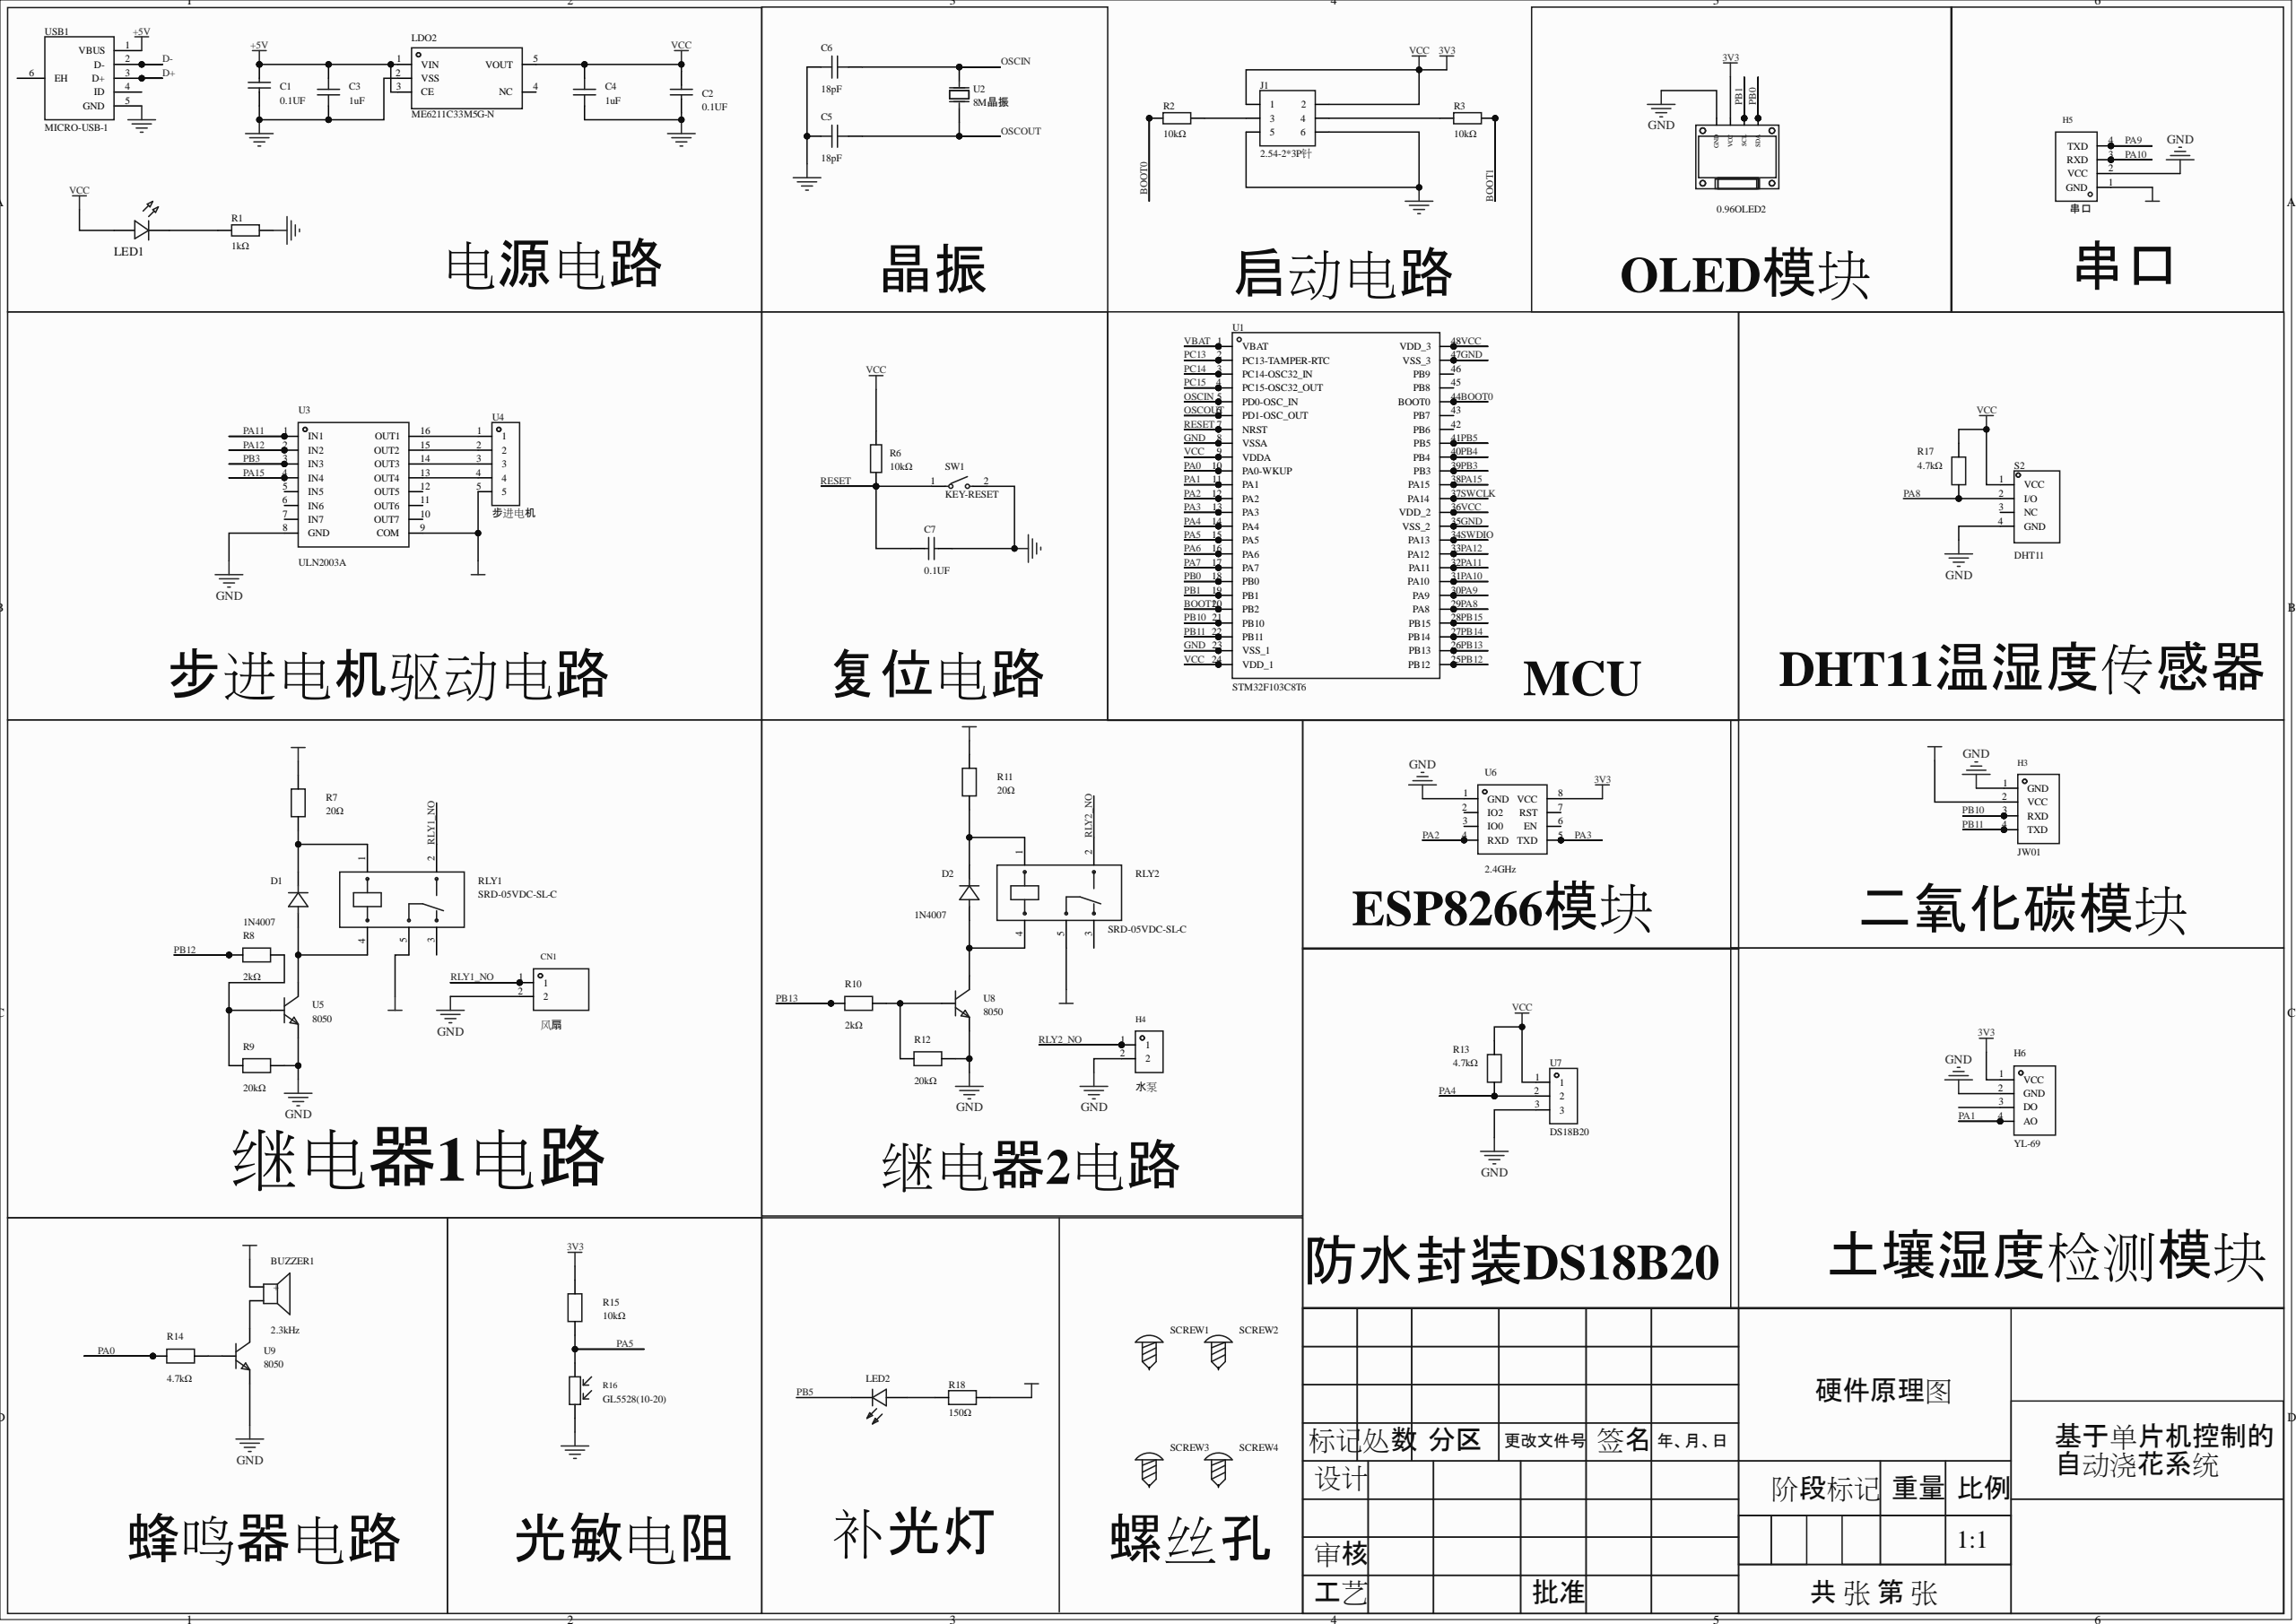Circuit board | Altium Designer | 54 parts | 46 nets
Bill of materials:
Comment,Description,Designator,Footprint,LibRef,Quantity
"","","0.96OLED2","oled-th_l27.8-w27.2-p2.54_c9900033791","0.96OLED模块_4P","1"
"2.3kHz","","BUZZER1","BUZ-TH_BD12.0-P7.60-D0.6-FD","TMB12A05_C96093","1"
"0.1UF","","C1, C2, C7","C0603","CAPCER0.1UF16VX5R0603,CAPCER0.1UF25VX5R0603,CAPCER0.1UF16VX7R0603","3"
"1uF","","C3, C4","C0603","TMK107B7105MA-T","2"
"18pF","","C5, C6","C0603","C1608C0G1H180J080AA","2"
"风扇","","CN1","CONN-TH_B2B-XH-A-LF-SN","B2B-XH-A(LF)(SN)","1"
"1N4007","","D1, D2","DO-41_BD2.4-L4.7-P8.70-D0.8-RD","1N4007_C2985028","2"
"JW01","","H3","HDR-TH_4P-P2.54-V-M","PZ254V-11-04P","1"
"水泵","","H4","HDR-TH_2P-P2.54-V-M","PZ254V-11-02P","1"
"串口","","H5","HDR-TH_4P-P2.54-V-M","PZ254V-11-04P","1"
"YL-69","","H6","HDR-TH_4P-P2.54-V-F","PM254V-11-04-H85","1"
"2.54-2*3P针","","J1","HDR-TH_6P-P2.54-V-M-R2-C3-S2.54-1","2.54-2*3P针","1"
"ME6211C33M5G-N","","LDO2","SOT-23-5_L3.0-W1.7-P0.95-LS2.8-BL","ME6211C33M5G-N","1"
"","","LED1","LED_0603","LED_0603-R","1"
"","","LED2","LED-TH_BD5.9-P2.54-RD","333-2SURD/S530-A3","1"
"1kΩ","","R1","R0603","0603WAF1001T5E","1"
"10kΩ","","R2, R3, R6","R0603","0603WAF1002T5E","3"
"20Ω","","R7, R11","RES-TH_BD2.3-L6.5-P10.50-D0.5","MF1/4W-1KΩ±1%T52","2"
"2kΩ","","R8, R10","RES-TH_BD2.3-L6.5-P10.50-D0.5","MF1/4W-1KΩ±1%T52","2"
"20kΩ","","R9, R12","RES-TH_BD2.3-L6.5-P10.50-D0.5","MF1/4W-1KΩ±1%T52","2"
"4.7kΩ","","R13, R14, R17","RES-TH_BD2.3-L6.5-P10.50-D0.5","MF1/4W-1KΩ±1%T52","3"
"10kΩ","","R15","RES-TH_BD2.3-L6.5-P10.50-D0.5","MF1/4W-1KΩ±1%T52","1"
"GL5528(10-20)","","R16","RES-TH_L5.1-W4.3-P3.40-D0.5","GL5528(10-20)_C10081","1"
"150Ω","","R18","RES-TH_BD2.3-L6.5-P10.50-D0.5","MF1/4W-1KΩ±1%T52","1"
"SRD-05VDC-SL-C","","RLY1, RLY2","RELAY-TH_SRD-XXVDC-XL-C","SRD-05VDC-SL-C","2"
"DHT11","","S2","SENSOR-TH_DHT11-1","DHT11_C87032","1"
"","","SCREW1, SCREW2, SCREW3, SCREW4","M2螺丝","M2螺丝","4"
"KEY-RESET","","SW1","SW-SMD_L6.0-W3.3-LS8.0","SW_PB2_A1","1"
"STM32F103C8T6","","U1","LQFP-48_L7.0-W7.0-P0.50-LS9.0-BL","STM32F103C8T6","1"
"8M晶振","","U2","HC-49S_L11.5-W4.7-P4.88","8M晶振_C9900011272","1"
"ULN2003A","","U3","DIP-16_L20.0-W6.4-P2.54-LS7.6-BL","ULN2003A_C93000","1"
"步进电机","","U4","CONN-TH_5P-P2.50_ZHOURI_XH-5PA","XH-5PA","1"
"8050","","U5, U8, U9","TO-92-3_L4.8-W3.7-P2.54-R","8050","3"
"2.4GHz","","U6","WIFIM-TH_8P-L24.7-W14.4-P2.54","ESP-01S","1"
"DS18B20","","U7","CONN-TH_3P-P5.00_KF301-5.0-3P","KF301-5.0-3P","1"
"MICRO-USB-1","","USB1","MICRO-USB-SMD_C9900008946","MICRO-USB-1","1"
Netlist (Protel format):
[
0.96OLED2
oled-th_l27.8-w27.2-p2.54_c9900033791




]
[
BUZZER1
BUZ-TH_BD12.0-P7.60-D0.6-FD
2.3kHz



]
[
C1
C0603
0.1UF



]
[
C2
C0603
0.1UF



]
[
C3
C0603
1uF



]
[
C4
C0603
1uF



]
[
C5
C0603
18pF



]
[
C6
C0603
18pF



]
[
C7
C0603
0.1UF



]
[
CN1
CONN-TH_B2B-XH-A-LF-SN
风扇



]
[
D1
DO-41_BD2.4-L4.7-P8.70-D0.8-RD
1N4007



]
[
D2
DO-41_BD2.4-L4.7-P8.70-D0.8-RD
1N4007



]
[
H3
HDR-TH_4P-P2.54-V-M
JW01



]
[
H4
HDR-TH_2P-P2.54-V-M
水泵



]
[
H5
HDR-TH_4P-P2.54-V-M
串口



]
[
H6
HDR-TH_4P-P2.54-V-F
YL-69



]
[
J1
HDR-TH_6P-P2.54-V-M-R2-C3-S2.54-1
2.54-2*3P针



]
[
LDO2
SOT-23-5_L3.0-W1.7-P0.95-LS2.8-BL
ME6211C33M5G-N



]
[
LED1
LED_0603




]
[
LED2
LED-TH_BD5.9-P2.54-RD




]
[
R1
R0603
1kΩ



]
[
R2
R0603
10kΩ



]
[
R3
R0603
10kΩ



]
[
R6
R0603
10kΩ



]
[
R7
RES-TH_BD2.3-L6.5-P10.50-D0.5
20Ω



]
[
R8
RES-TH_BD2.3-L6.5-P10.50-D0.5
2kΩ



]
[
R9
RES-TH_BD2.3-L6.5-P10.50-D0.5
20kΩ



]
[
R10
RES-TH_BD2.3-L6.5-P10.50-D0.5
2kΩ



]
[
R11
RES-TH_BD2.3-L6.5-P10.50-D0.5
20Ω



]
[
R12
RES-TH_BD2.3-L6.5-P10.50-D0.5
20kΩ



]
[
R13
RES-TH_BD2.3-L6.5-P10.50-D0.5
4.7kΩ



]
[
R14
RES-TH_BD2.3-L6.5-P10.50-D0.5
4.7kΩ



]
[
R15
RES-TH_BD2.3-L6.5-P10.50-D0.5
10kΩ



]
[
R16
RES-TH_L5.1-W4.3-P3.40-D0.5
GL5528(10-20)



]
[
R17
RES-TH_BD2.3-L6.5-P10.50-D0.5
4.7kΩ



]
[
R18
RES-TH_BD2.3-L6.5-P10.50-D0.5
150Ω



]
[
RLY1
RELAY-TH_SRD-XXVDC-XL-C
SRD-05VDC-SL-C



]
[
RLY2
RELAY-TH_SRD-XXVDC-XL-C
SRD-05VDC-SL-C



]
[
S2
SENSOR-TH_DHT11-1
DHT11



]
[
SCREW1
M2螺丝




]
[
SCREW2
M2螺丝




]
[
SCREW3
M2螺丝




]
[
SCREW4
M2螺丝




]
[
SW1
SW-SMD_L6.0-W3.3-LS8.0
KEY-RESET



]
[
U1
LQFP-48_L7.0-W7.0-P0.50-LS9.0-BL
STM32F103C8T6



]
[
U2
HC-49S_L11.5-W4.7-P4.88
8M晶振



]
[
U3
DIP-16_L20.0-W6.4-P2.54-LS7.6-BL
ULN2003A



]
[
U4
CONN-TH_5P-P2.50_ZHOURI_XH-5PA
步进电机



]
[
U5
TO-92-3_L4.8-W3.7-P2.54-R
8050



]
[
U6
WIFIM-TH_8P-L24.7-W14.4-P2.54
2.4GHz



]
[
U7
CONN-TH_3P-P5.00_KF301-5.0-3P
DS18B20



]
[
U8
TO-92-3_L4.8-W3.7-P2.54-R
8050



]
[
U9
TO-92-3_L4.8-W3.7-P2.54-R
8050



]
[
USB1
MICRO-USB-SMD_C9900008946
MICRO-USB-1



]
(
VCC
0.96OLED2-2
BUZZER1-1
C2-2
C4-2
H3-2
H5-1
H6-1
J1-1
J1-2
LDO2-5
LED1-2
R6-2
R7-2
R11-2
R13-2
R15-2
R17-2
R18-2
RLY1-5
RLY2-5
S2-1
U1-9
U1-24
U1-36
U1-48
U3-9
U4-5
U6-8
U7-1
)
(
RLY2_NO
H4-1
RLY2-2
)
(
RLY1_NO
CN1-1
RLY1-2
)
(
RESET
C7-1
R6-1
SW1-1
U1-7
)
(
PB13
R10-1
U1-26
)
(
PB12
R8-1
U1-25
)
(
PB11
H3-4
U1-22
)
(
PB10
H3-3
U1-21
)
(
PB5
LED2-1
U1-41
)
(
PB3
U1-39
U3-3
)
(
PB1
0.96OLED2-3
U1-19
)
(
PB0
0.96OLED2-4
U1-18
)
(
PA15
U1-38
U3-4
)
(
PA12
U1-33
U3-2
)
(
PA11
U1-32
U3-1
)
(
PA10
H5-3
U1-31
)
(
PA9
H5-4
U1-30
)
(
PA8
R17-1
S2-2
U1-29
)
(
PA5
R15-1
R16-1
U1-15
)
(
PA4
R13-1
U1-14
U7-2
)
(
PA3
U1-13
U6-5
)
(
PA2
U1-12
U6-4
)
(
PA1
H6-4
U1-11
)
(
PA0
R14-1
U1-10
)
(
OSCOUT
C5-1
U1-6
U2-2
)
(
OSCIN
C6-2
U1-5
U2-1
)
(
NetU3_16
U3-16
U4-1
)
(
NetU3_15
U3-15
U4-2
)
(
NetU3_14
U3-14
U4-3
)
(
NetU3_13
U3-13
U4-4
)
(
NetR14_2
R14-2
U9-2
)
(
NetR10_2
R10-2
R12-1
U8-2
)
(
NetR8_2
R8-2
R9-1
U5-2
)
(
NetLED2_2
LED2-2
R18-1
)
(
NetLED1_1
LED1-1
R1-1
)
(
NetJ1_4
J1-4
R3-1
)
(
NetJ1_3
J1-3
R2-2
)
(
NetD2_2
D2-2
RLY2-4
U8-1
)
(
NetD2_1
D2-1
R11-1
RLY2-1
)
(
NetD1_2
D1-2
RLY1-4
U5-1
)
(
NetD1_1
D1-1
R7-1
RLY1-1
)
(
NetBUZZER1_2
BUZZER1-2
U9-1
)
(
GND
0.96OLED2-1
C1-1
C2-1
C3-1
C4-1
C5-2
C6-1
C7-2
CN1-2
H3-1
H4-2
H5-2
H6-2
J1-5
J1-6
LDO2-2
R1-2
R9-2
R12-2
R16-2
S2-4
SW1-2
U1-8
U1-23
U1-35
U1-47
U3-8
U5-3
U6-1
U7-3
U8-3
U9-3
USB1-5
)
(
BOOT1
R3-2
U1-20
)
(
BOOT0
R2-1
U1-44
)
(
+5V
C1-2
C3-2
LDO2-1
LDO2-3
USB1-1
)